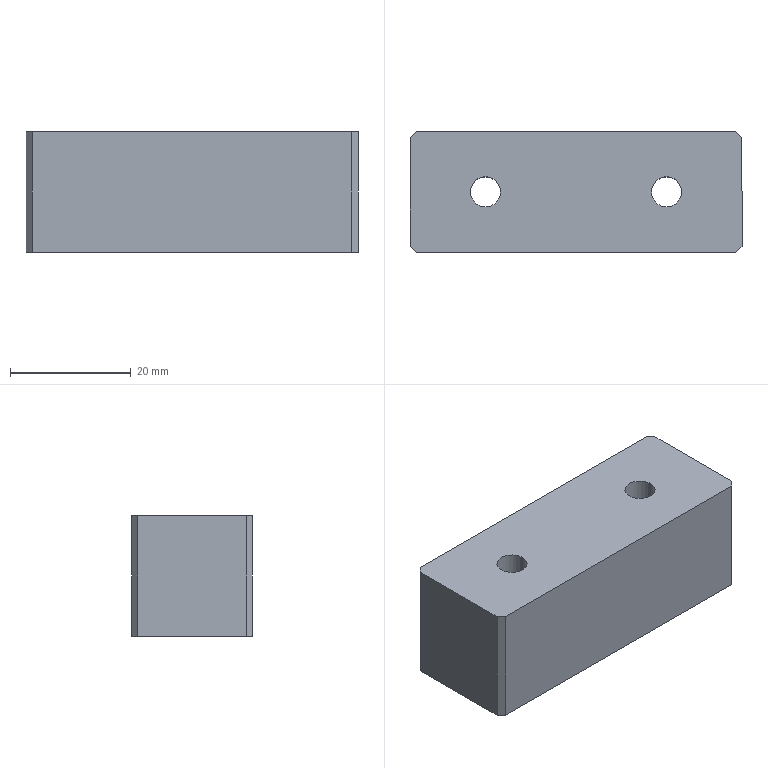Part | SolidWorks | features Chamfer 1, Extrusion 1, HoleWzd 1 | 1 solid | 14 faces | box 55 x 20 x 20 mm | volume 21175 mm3 | plane 10 | cylinder 4 | commonest cylinder face diameters 5 x4
STEP:
#1=CARTESIAN_POINT('',(-69.836,28.056,0.));
#2=VERTEX_POINT('',#1);
#3=CARTESIAN_POINT('',(-64.836,28.056,0.));
#4=VERTEX_POINT('',#3);
#5=CARTESIAN_POINT('',(-67.336,28.056,0.));
#6=DIRECTION('',(0.,0.,1.));
#7=DIRECTION('',(1.,0.,0.));
#8=AXIS2_PLACEMENT_3D('',#5,#6,#7);
#9=CIRCLE('',#8,2.5);
#10=EDGE_CURVE('',#2,#4,#9,.T.);
#11=ORIENTED_EDGE('',*,*,#10,.F.);
#12=CARTESIAN_POINT('',(-69.836,28.056,20.));
#13=VERTEX_POINT('',#12);
#14=CARTESIAN_POINT('',(-69.836,28.056,20.));
#15=DIRECTION('',(0.,0.,1.));
#16=VECTOR('',#15,1000.);
#17=LINE('',#14,#16);
#18=EDGE_CURVE('',#2,#13,#17,.T.);
#19=ORIENTED_EDGE('',*,*,#18,.T.);
#20=CARTESIAN_POINT('',(-64.836,28.056,20.));
#21=VERTEX_POINT('',#20);
#22=CARTESIAN_POINT('',(-67.336,28.056,20.));
#23=DIRECTION('',(0.,0.,1.));
#24=DIRECTION('',(1.,0.,0.));
#25=AXIS2_PLACEMENT_3D('',#22,#23,#24);
#26=CIRCLE('',#25,2.5);
#27=EDGE_CURVE('',#13,#21,#26,.T.);
#28=ORIENTED_EDGE('',*,*,#27,.T.);
#29=CARTESIAN_POINT('',(-64.836,28.056,20.));
#30=DIRECTION('',(0.,0.,1.));
#31=VECTOR('',#30,1000.);
#32=LINE('',#29,#31);
#33=EDGE_CURVE('',#4,#21,#32,.T.);
#34=ORIENTED_EDGE('',*,*,#33,.F.);
#35=EDGE_LOOP('',(#11,#19,#28,#34));
#36=FACE_OUTER_BOUND('',#35,.T.);
#37=CARTESIAN_POINT('',(-67.336,28.056,20.));
#38=DIRECTION('',(0.,0.,1.));
#39=DIRECTION('',(1.,0.,0.));
#40=AXIS2_PLACEMENT_3D('',#37,#38,#39);
#41=CYLINDRICAL_SURFACE('',#40,2.5);
#42=ADVANCED_FACE('',(#36),#41,.F.);
#43=CARTESIAN_POINT('',(-39.836,28.056,0.));
#44=VERTEX_POINT('',#43);
#45=CARTESIAN_POINT('',(-34.836,28.056,0.));
#46=VERTEX_POINT('',#45);
#47=CARTESIAN_POINT('',(-37.336,28.056,0.));
#48=DIRECTION('',(0.,0.,1.));
#49=DIRECTION('',(1.,0.,0.));
#50=AXIS2_PLACEMENT_3D('',#47,#48,#49);
#51=CIRCLE('',#50,2.5);
#52=EDGE_CURVE('',#44,#46,#51,.T.);
#53=ORIENTED_EDGE('',*,*,#52,.F.);
#54=CARTESIAN_POINT('',(-39.836,28.056,20.));
#55=VERTEX_POINT('',#54);
#56=CARTESIAN_POINT('',(-39.836,28.056,20.));
#57=DIRECTION('',(0.,0.,1.));
#58=VECTOR('',#57,1000.);
#59=LINE('',#56,#58);
#60=EDGE_CURVE('',#44,#55,#59,.T.);
#61=ORIENTED_EDGE('',*,*,#60,.T.);
#62=CARTESIAN_POINT('',(-34.836,28.056,20.));
#63=VERTEX_POINT('',#62);
#64=CARTESIAN_POINT('',(-37.336,28.056,20.));
#65=DIRECTION('',(0.,0.,1.));
#66=DIRECTION('',(1.,0.,0.));
#67=AXIS2_PLACEMENT_3D('',#64,#65,#66);
#68=CIRCLE('',#67,2.5);
#69=EDGE_CURVE('',#55,#63,#68,.T.);
#70=ORIENTED_EDGE('',*,*,#69,.T.);
#71=CARTESIAN_POINT('',(-34.836,28.056,20.));
#72=DIRECTION('',(0.,0.,1.));
#73=VECTOR('',#72,1000.);
#74=LINE('',#71,#73);
#75=EDGE_CURVE('',#46,#63,#74,.T.);
#76=ORIENTED_EDGE('',*,*,#75,.F.);
#77=EDGE_LOOP('',(#53,#61,#70,#76));
#78=FACE_OUTER_BOUND('',#77,.T.);
#79=CARTESIAN_POINT('',(-37.336,28.056,20.));
#80=DIRECTION('',(0.,0.,1.));
#81=DIRECTION('',(1.,0.,0.));
#82=AXIS2_PLACEMENT_3D('',#79,#80,#81);
#83=CYLINDRICAL_SURFACE('',#82,2.5);
#84=ADVANCED_FACE('',(#78),#83,.F.);
#85=CARTESIAN_POINT('',(-79.836,37.056,0.));
#86=VERTEX_POINT('',#85);
#87=CARTESIAN_POINT('',(-79.836,19.056,0.));
#88=VERTEX_POINT('',#87);
#89=CARTESIAN_POINT('',(-79.836,38.056,0.));
#90=DIRECTION('',(0.,-1.,0.));
#91=VECTOR('',#90,1000.);
#92=LINE('',#89,#91);
#93=EDGE_CURVE('',#86,#88,#92,.T.);
#94=ORIENTED_EDGE('',*,*,#93,.T.);
#95=CARTESIAN_POINT('',(-79.836,19.056,20.));
#96=VERTEX_POINT('',#95);
#97=CARTESIAN_POINT('',(-79.836,19.056,20.));
#98=DIRECTION('',(0.,0.,1.));
#99=VECTOR('',#98,1000.);
#100=LINE('',#97,#99);
#101=EDGE_CURVE('',#88,#96,#100,.T.);
#102=ORIENTED_EDGE('',*,*,#101,.T.);
#103=CARTESIAN_POINT('',(-79.836,37.056,20.));
#104=VERTEX_POINT('',#103);
#105=CARTESIAN_POINT('',(-79.836,38.056,20.));
#106=DIRECTION('',(0.,-1.,0.));
#107=VECTOR('',#106,1000.);
#108=LINE('',#105,#107);
#109=EDGE_CURVE('',#104,#96,#108,.T.);
#110=ORIENTED_EDGE('',*,*,#109,.F.);
#111=CARTESIAN_POINT('',(-79.836,37.056,20.));
#112=DIRECTION('',(0.,0.,-1.));
#113=VECTOR('',#112,1000.);
#114=LINE('',#111,#113);
#115=EDGE_CURVE('',#104,#86,#114,.T.);
#116=ORIENTED_EDGE('',*,*,#115,.T.);
#117=EDGE_LOOP('',(#94,#102,#110,#116));
#118=FACE_OUTER_BOUND('',#117,.T.);
#119=CARTESIAN_POINT('',(-79.836,38.056,20.));
#120=DIRECTION('',(1.,0.,0.));
#121=DIRECTION('',(0.,1.,0.));
#122=AXIS2_PLACEMENT_3D('',#119,#120,#121);
#123=PLANE('',#122);
#124=ADVANCED_FACE('',(#118),#123,.F.);
#125=CARTESIAN_POINT('',(-78.836,18.056,0.));
#126=VERTEX_POINT('',#125);
#127=CARTESIAN_POINT('',(-25.836,18.056,0.));
#128=VERTEX_POINT('',#127);
#129=CARTESIAN_POINT('',(-79.836,18.056,0.));
#130=DIRECTION('',(1.,0.,0.));
#131=VECTOR('',#130,1000.);
#132=LINE('',#129,#131);
#133=EDGE_CURVE('',#126,#128,#132,.T.);
#134=ORIENTED_EDGE('',*,*,#133,.T.);
#135=CARTESIAN_POINT('',(-25.836,18.056,20.));
#136=VERTEX_POINT('',#135);
#137=CARTESIAN_POINT('',(-25.836,18.056,20.));
#138=DIRECTION('',(0.,0.,1.));
#139=VECTOR('',#138,1000.);
#140=LINE('',#137,#139);
#141=EDGE_CURVE('',#128,#136,#140,.T.);
#142=ORIENTED_EDGE('',*,*,#141,.T.);
#143=CARTESIAN_POINT('',(-78.836,18.056,20.));
#144=VERTEX_POINT('',#143);
#145=CARTESIAN_POINT('',(-79.836,18.056,20.));
#146=DIRECTION('',(1.,0.,0.));
#147=VECTOR('',#146,1000.);
#148=LINE('',#145,#147);
#149=EDGE_CURVE('',#144,#136,#148,.T.);
#150=ORIENTED_EDGE('',*,*,#149,.F.);
#151=CARTESIAN_POINT('',(-78.836,18.056,20.));
#152=DIRECTION('',(0.,0.,-1.));
#153=VECTOR('',#152,1000.);
#154=LINE('',#151,#153);
#155=EDGE_CURVE('',#144,#126,#154,.T.);
#156=ORIENTED_EDGE('',*,*,#155,.T.);
#157=EDGE_LOOP('',(#134,#142,#150,#156));
#158=FACE_OUTER_BOUND('',#157,.T.);
#159=CARTESIAN_POINT('',(-79.836,18.056,20.));
#160=DIRECTION('',(0.,1.,0.));
#161=DIRECTION('',(0.,0.,1.));
#162=AXIS2_PLACEMENT_3D('',#159,#160,#161);
#163=PLANE('',#162);
#164=ADVANCED_FACE('',(#158),#163,.F.);
#165=CARTESIAN_POINT('',(-24.836,19.056,0.));
#166=VERTEX_POINT('',#165);
#167=CARTESIAN_POINT('',(-24.836,37.056,0.));
#168=VERTEX_POINT('',#167);
#169=CARTESIAN_POINT('',(-24.836,38.056,0.));
#170=DIRECTION('',(0.,1.,0.));
#171=VECTOR('',#170,1000.);
#172=LINE('',#169,#171);
#173=EDGE_CURVE('',#166,#168,#172,.T.);
#174=ORIENTED_EDGE('',*,*,#173,.T.);
#175=CARTESIAN_POINT('',(-24.836,37.056,20.));
#176=VERTEX_POINT('',#175);
#177=CARTESIAN_POINT('',(-24.836,37.056,20.));
#178=DIRECTION('',(0.,0.,1.));
#179=VECTOR('',#178,1000.);
#180=LINE('',#177,#179);
#181=EDGE_CURVE('',#168,#176,#180,.T.);
#182=ORIENTED_EDGE('',*,*,#181,.T.);
#183=CARTESIAN_POINT('',(-24.836,19.056,20.));
#184=VERTEX_POINT('',#183);
#185=CARTESIAN_POINT('',(-24.836,38.056,20.));
#186=DIRECTION('',(0.,1.,0.));
#187=VECTOR('',#186,1000.);
#188=LINE('',#185,#187);
#189=EDGE_CURVE('',#184,#176,#188,.T.);
#190=ORIENTED_EDGE('',*,*,#189,.F.);
#191=CARTESIAN_POINT('',(-24.836,19.056,20.));
#192=DIRECTION('',(0.,0.,-1.));
#193=VECTOR('',#192,1000.);
#194=LINE('',#191,#193);
#195=EDGE_CURVE('',#184,#166,#194,.T.);
#196=ORIENTED_EDGE('',*,*,#195,.T.);
#197=EDGE_LOOP('',(#174,#182,#190,#196));
#198=FACE_OUTER_BOUND('',#197,.T.);
#199=CARTESIAN_POINT('',(-24.836,38.056,20.));
#200=DIRECTION('',(-1.,0.,0.));
#201=DIRECTION('',(0.,-1.,0.));
#202=AXIS2_PLACEMENT_3D('',#199,#200,#201);
#203=PLANE('',#202);
#204=ADVANCED_FACE('',(#198),#203,.F.);
#205=CARTESIAN_POINT('',(-25.836,38.056,20.));
#206=VERTEX_POINT('',#205);
#207=CARTESIAN_POINT('',(-78.836,38.056,20.));
#208=VERTEX_POINT('',#207);
#209=CARTESIAN_POINT('',(-79.836,38.056,20.));
#210=DIRECTION('',(-1.,0.,0.));
#211=VECTOR('',#210,1000.);
#212=LINE('',#209,#211);
#213=EDGE_CURVE('',#206,#208,#212,.T.);
#214=ORIENTED_EDGE('',*,*,#213,.F.);
#215=CARTESIAN_POINT('',(-25.836,38.056,0.));
#216=VERTEX_POINT('',#215);
#217=CARTESIAN_POINT('',(-25.836,38.056,20.));
#218=DIRECTION('',(0.,0.,-1.));
#219=VECTOR('',#218,1000.);
#220=LINE('',#217,#219);
#221=EDGE_CURVE('',#206,#216,#220,.T.);
#222=ORIENTED_EDGE('',*,*,#221,.T.);
#223=CARTESIAN_POINT('',(-78.836,38.056,0.));
#224=VERTEX_POINT('',#223);
#225=CARTESIAN_POINT('',(-79.836,38.056,0.));
#226=DIRECTION('',(-1.,0.,0.));
#227=VECTOR('',#226,1000.);
#228=LINE('',#225,#227);
#229=EDGE_CURVE('',#216,#224,#228,.T.);
#230=ORIENTED_EDGE('',*,*,#229,.T.);
#231=CARTESIAN_POINT('',(-78.836,38.056,20.));
#232=DIRECTION('',(0.,0.,1.));
#233=VECTOR('',#232,1000.);
#234=LINE('',#231,#233);
#235=EDGE_CURVE('',#224,#208,#234,.T.);
#236=ORIENTED_EDGE('',*,*,#235,.T.);
#237=EDGE_LOOP('',(#214,#222,#230,#236));
#238=FACE_OUTER_BOUND('',#237,.T.);
#239=CARTESIAN_POINT('',(-79.836,38.056,20.));
#240=DIRECTION('',(0.,-1.,0.));
#241=DIRECTION('',(0.,0.,-1.));
#242=AXIS2_PLACEMENT_3D('',#239,#240,#241);
#243=PLANE('',#242);
#244=ADVANCED_FACE('',(#238),#243,.F.);
#245=CARTESIAN_POINT('',(-67.336,28.056,20.));
#246=DIRECTION('',(0.,0.,1.));
#247=DIRECTION('',(1.,0.,0.));
#248=AXIS2_PLACEMENT_3D('',#245,#246,#247);
#249=CIRCLE('',#248,2.5);
#250=EDGE_CURVE('',#21,#13,#249,.T.);
#251=ORIENTED_EDGE('',*,*,#250,.F.);
#252=ORIENTED_EDGE('',*,*,#27,.F.);
#253=EDGE_LOOP('',(#251,#252));
#254=FACE_BOUND('',#253,.T.);
#255=CARTESIAN_POINT('',(-37.336,28.056,20.));
#256=DIRECTION('',(0.,0.,1.));
#257=DIRECTION('',(1.,0.,0.));
#258=AXIS2_PLACEMENT_3D('',#255,#256,#257);
#259=CIRCLE('',#258,2.5);
#260=EDGE_CURVE('',#63,#55,#259,.T.);
#261=ORIENTED_EDGE('',*,*,#260,.F.);
#262=ORIENTED_EDGE('',*,*,#69,.F.);
#263=EDGE_LOOP('',(#261,#262));
#264=FACE_BOUND('',#263,.T.);
#265=ORIENTED_EDGE('',*,*,#189,.T.);
#266=CARTESIAN_POINT('',(6.11,6.11,20.));
#267=DIRECTION('',(-0.7071,0.7071,0.));
#268=VECTOR('',#267,1000.);
#269=LINE('',#266,#268);
#270=EDGE_CURVE('',#176,#206,#269,.T.);
#271=ORIENTED_EDGE('',*,*,#270,.T.);
#272=ORIENTED_EDGE('',*,*,#213,.T.);
#273=CARTESIAN_POINT('',(-58.446,58.446,20.));
#274=DIRECTION('',(-0.7071,-0.7071,0.));
#275=VECTOR('',#274,1000.);
#276=LINE('',#273,#275);
#277=EDGE_CURVE('',#208,#104,#276,.T.);
#278=ORIENTED_EDGE('',*,*,#277,.T.);
#279=ORIENTED_EDGE('',*,*,#109,.T.);
#280=CARTESIAN_POINT('',(-30.39,-30.39,20.));
#281=DIRECTION('',(0.7071,-0.7071,0.));
#282=VECTOR('',#281,1000.);
#283=LINE('',#280,#282);
#284=EDGE_CURVE('',#96,#144,#283,.T.);
#285=ORIENTED_EDGE('',*,*,#284,.T.);
#286=ORIENTED_EDGE('',*,*,#149,.T.);
#287=CARTESIAN_POINT('',(-21.946,21.946,20.));
#288=DIRECTION('',(0.7071,0.7071,0.));
#289=VECTOR('',#288,1000.);
#290=LINE('',#287,#289);
#291=EDGE_CURVE('',#136,#184,#290,.T.);
#292=ORIENTED_EDGE('',*,*,#291,.T.);
#293=EDGE_LOOP('',(#265,#271,#272,#278,#279,#285,#286,#292));
#294=FACE_OUTER_BOUND('',#293,.T.);
#295=CARTESIAN_POINT('',(0.,0.,20.));
#296=DIRECTION('',(0.,0.,1.));
#297=DIRECTION('',(1.,0.,0.));
#298=AXIS2_PLACEMENT_3D('',#295,#296,#297);
#299=PLANE('',#298);
#300=ADVANCED_FACE('',(#254,#264,#294),#299,.T.);
#301=CARTESIAN_POINT('',(-67.336,28.056,0.));
#302=DIRECTION('',(0.,0.,1.));
#303=DIRECTION('',(1.,0.,0.));
#304=AXIS2_PLACEMENT_3D('',#301,#302,#303);
#305=CIRCLE('',#304,2.5);
#306=EDGE_CURVE('',#4,#2,#305,.T.);
#307=ORIENTED_EDGE('',*,*,#306,.T.);
#308=ORIENTED_EDGE('',*,*,#10,.T.);
#309=EDGE_LOOP('',(#307,#308));
#310=FACE_BOUND('',#309,.T.);
#311=CARTESIAN_POINT('',(-37.336,28.056,0.));
#312=DIRECTION('',(0.,0.,1.));
#313=DIRECTION('',(1.,0.,0.));
#314=AXIS2_PLACEMENT_3D('',#311,#312,#313);
#315=CIRCLE('',#314,2.5);
#316=EDGE_CURVE('',#46,#44,#315,.T.);
#317=ORIENTED_EDGE('',*,*,#316,.T.);
#318=ORIENTED_EDGE('',*,*,#52,.T.);
#319=EDGE_LOOP('',(#317,#318));
#320=FACE_BOUND('',#319,.T.);
#321=ORIENTED_EDGE('',*,*,#229,.F.);
#322=CARTESIAN_POINT('',(-25.836,38.056,0.));
#323=DIRECTION('',(0.7071,-0.7071,0.));
#324=VECTOR('',#323,1000.);
#325=LINE('',#322,#324);
#326=EDGE_CURVE('',#216,#168,#325,.T.);
#327=ORIENTED_EDGE('',*,*,#326,.T.);
#328=ORIENTED_EDGE('',*,*,#173,.F.);
#329=CARTESIAN_POINT('',(-24.836,19.056,0.));
#330=DIRECTION('',(-0.7071,-0.7071,0.));
#331=VECTOR('',#330,1000.);
#332=LINE('',#329,#331);
#333=EDGE_CURVE('',#166,#128,#332,.T.);
#334=ORIENTED_EDGE('',*,*,#333,.T.);
#335=ORIENTED_EDGE('',*,*,#133,.F.);
#336=CARTESIAN_POINT('',(-78.836,18.056,0.));
#337=DIRECTION('',(-0.7071,0.7071,0.));
#338=VECTOR('',#337,1000.);
#339=LINE('',#336,#338);
#340=EDGE_CURVE('',#126,#88,#339,.T.);
#341=ORIENTED_EDGE('',*,*,#340,.T.);
#342=ORIENTED_EDGE('',*,*,#93,.F.);
#343=CARTESIAN_POINT('',(-79.836,37.056,0.));
#344=DIRECTION('',(0.7071,0.7071,0.));
#345=VECTOR('',#344,1000.);
#346=LINE('',#343,#345);
#347=EDGE_CURVE('',#86,#224,#346,.T.);
#348=ORIENTED_EDGE('',*,*,#347,.T.);
#349=EDGE_LOOP('',(#321,#327,#328,#334,#335,#341,#342,#348));
#350=FACE_OUTER_BOUND('',#349,.T.);
#351=CARTESIAN_POINT('',(0.,0.,0.));
#352=DIRECTION('',(0.,0.,1.));
#353=DIRECTION('',(1.,0.,0.));
#354=AXIS2_PLACEMENT_3D('',#351,#352,#353);
#355=PLANE('',#354);
#356=ADVANCED_FACE('',(#310,#320,#350),#355,.F.);
#357=ORIENTED_EDGE('',*,*,#60,.F.);
#358=ORIENTED_EDGE('',*,*,#316,.F.);
#359=ORIENTED_EDGE('',*,*,#75,.T.);
#360=ORIENTED_EDGE('',*,*,#260,.T.);
#361=EDGE_LOOP('',(#357,#358,#359,#360));
#362=FACE_OUTER_BOUND('',#361,.T.);
#363=CARTESIAN_POINT('',(-37.336,28.056,20.));
#364=DIRECTION('',(0.,0.,1.));
#365=DIRECTION('',(1.,0.,0.));
#366=AXIS2_PLACEMENT_3D('',#363,#364,#365);
#367=CYLINDRICAL_SURFACE('',#366,2.5);
#368=ADVANCED_FACE('',(#362),#367,.F.);
#369=ORIENTED_EDGE('',*,*,#18,.F.);
#370=ORIENTED_EDGE('',*,*,#306,.F.);
#371=ORIENTED_EDGE('',*,*,#33,.T.);
#372=ORIENTED_EDGE('',*,*,#250,.T.);
#373=EDGE_LOOP('',(#369,#370,#371,#372));
#374=FACE_OUTER_BOUND('',#373,.T.);
#375=CARTESIAN_POINT('',(-67.336,28.056,20.));
#376=DIRECTION('',(0.,0.,1.));
#377=DIRECTION('',(1.,0.,0.));
#378=AXIS2_PLACEMENT_3D('',#375,#376,#377);
#379=CYLINDRICAL_SURFACE('',#378,2.5);
#380=ADVANCED_FACE('',(#374),#379,.F.);
#381=ORIENTED_EDGE('',*,*,#270,.F.);
#382=ORIENTED_EDGE('',*,*,#181,.F.);
#383=ORIENTED_EDGE('',*,*,#326,.F.);
#384=ORIENTED_EDGE('',*,*,#221,.F.);
#385=EDGE_LOOP('',(#381,#382,#383,#384));
#386=FACE_OUTER_BOUND('',#385,.T.);
#387=CARTESIAN_POINT('',(-25.836,38.056,20.));
#388=DIRECTION('',(-0.7071,-0.7071,0.));
#389=DIRECTION('',(0.,0.,-1.));
#390=AXIS2_PLACEMENT_3D('',#387,#388,#389);
#391=PLANE('',#390);
#392=ADVANCED_FACE('',(#386),#391,.F.);
#393=ORIENTED_EDGE('',*,*,#291,.F.);
#394=ORIENTED_EDGE('',*,*,#141,.F.);
#395=ORIENTED_EDGE('',*,*,#333,.F.);
#396=ORIENTED_EDGE('',*,*,#195,.F.);
#397=EDGE_LOOP('',(#393,#394,#395,#396));
#398=FACE_OUTER_BOUND('',#397,.T.);
#399=CARTESIAN_POINT('',(-24.836,19.056,20.));
#400=DIRECTION('',(-0.7071,0.7071,0.));
#401=DIRECTION('',(0.,0.,-1.));
#402=AXIS2_PLACEMENT_3D('',#399,#400,#401);
#403=PLANE('',#402);
#404=ADVANCED_FACE('',(#398),#403,.F.);
#405=ORIENTED_EDGE('',*,*,#284,.F.);
#406=ORIENTED_EDGE('',*,*,#101,.F.);
#407=ORIENTED_EDGE('',*,*,#340,.F.);
#408=ORIENTED_EDGE('',*,*,#155,.F.);
#409=EDGE_LOOP('',(#405,#406,#407,#408));
#410=FACE_OUTER_BOUND('',#409,.T.);
#411=CARTESIAN_POINT('',(-78.836,18.056,20.));
#412=DIRECTION('',(0.7071,0.7071,0.));
#413=DIRECTION('',(0.,0.,-1.));
#414=AXIS2_PLACEMENT_3D('',#411,#412,#413);
#415=PLANE('',#414);
#416=ADVANCED_FACE('',(#410),#415,.F.);
#417=ORIENTED_EDGE('',*,*,#277,.F.);
#418=ORIENTED_EDGE('',*,*,#235,.F.);
#419=ORIENTED_EDGE('',*,*,#347,.F.);
#420=ORIENTED_EDGE('',*,*,#115,.F.);
#421=EDGE_LOOP('',(#417,#418,#419,#420));
#422=FACE_OUTER_BOUND('',#421,.T.);
#423=CARTESIAN_POINT('',(-79.836,37.056,20.));
#424=DIRECTION('',(0.7071,-0.7071,0.));
#425=DIRECTION('',(0.,0.,-1.));
#426=AXIS2_PLACEMENT_3D('',#423,#424,#425);
#427=PLANE('',#426);
#428=ADVANCED_FACE('',(#422),#427,.F.);
#429=CLOSED_SHELL('',(#42,#84,#124,#164,#204,#244,#300,#356,#368,#380,#392,#404,#416,#428));
#430=MANIFOLD_SOLID_BREP('',#429);
#431=CARTESIAN_POINT('',(0.,0.,0.));
#432=DIRECTION('',(0.,0.,1.));
#433=DIRECTION('',(1.,0.,0.));
#434=AXIS2_PLACEMENT_3D('',#431,#432,#433);
#435=(LENGTH_UNIT()NAMED_UNIT(*)SI_UNIT(.MILLI.,.METRE.));
#436=UNCERTAINTY_MEASURE_WITH_UNIT(LENGTH_MEASURE(0.00001),#435,'','');
#437=(NAMED_UNIT(*)PLANE_ANGLE_UNIT()SI_UNIT($,.RADIAN.));
#438=(NAMED_UNIT(*)SI_UNIT($,.STERADIAN.)SOLID_ANGLE_UNIT());
#439=(GEOMETRIC_REPRESENTATION_CONTEXT(3)GLOBAL_UNCERTAINTY_ASSIGNED_CONTEXT((#436))GLOBAL_UNIT_ASSIGNED_CONTEXT((#435,#437,#438))REPRESENTATION_CONTEXT('',''));
#440=ADVANCED_BREP_SHAPE_REPRESENTATION('',(#430,#434),#439);